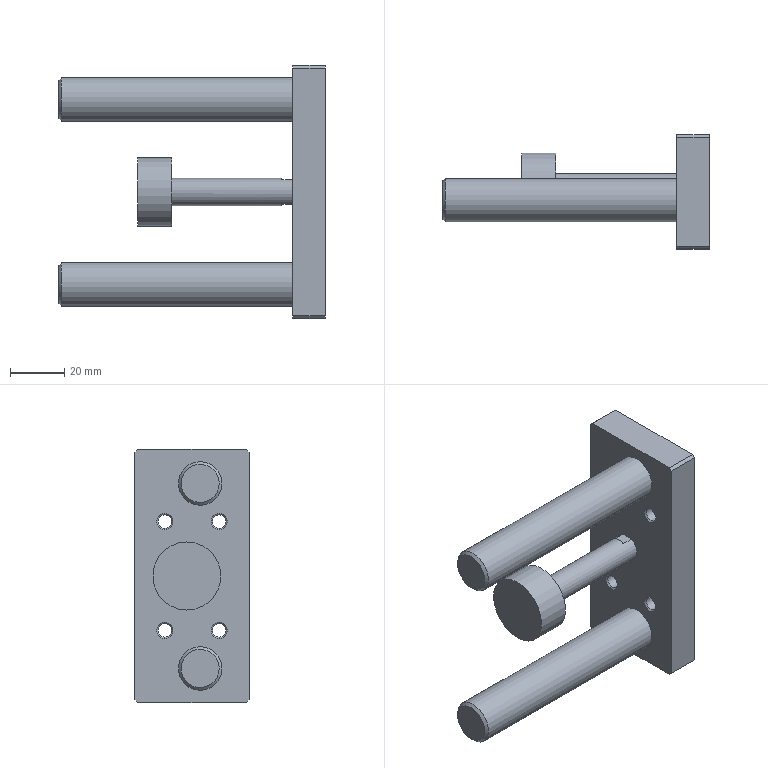Part | NX | features BREP 1 | 1 solid | 102 faces | box 98 x 42 x 93 mm | volume 89310 mm3 | cylinder 54 | plane 31 | cone 14 | torus 3 | commonest cylinder face diameters 1.12 x18 1.96 x18 4.917 x4 9 x4 10 x4 11 x3